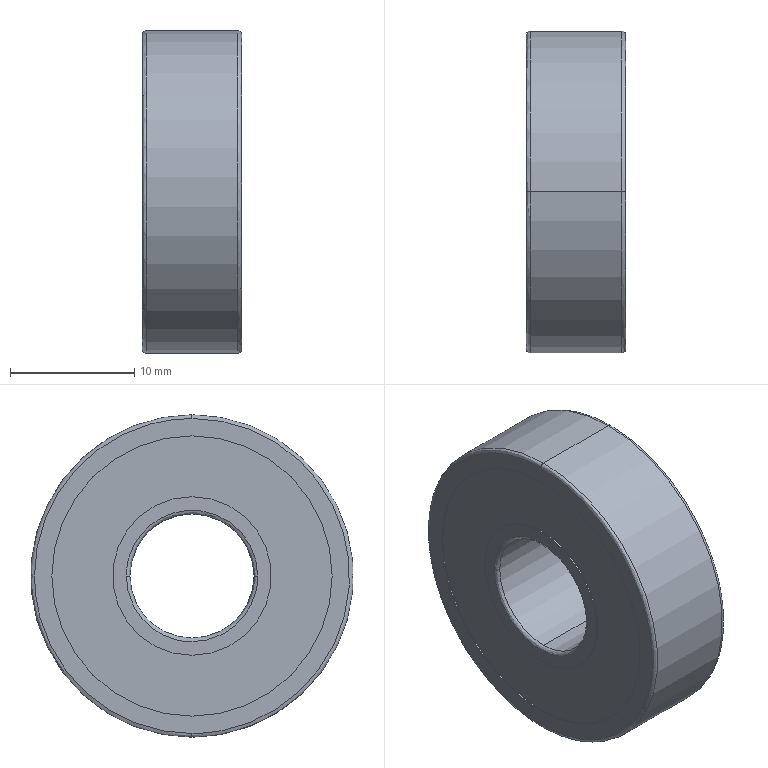Part | STEP file | TQ-DD-1105-TH 6000ZZ_2_031010 Default | 13 solids | 90 faces | box 8 x 26 x 26 mm | volume 2409 mm3 | spline 50 | cylinder 28 | plane 12 | commonest cylinder face diameters 12.8 x8 22.6 x8 14.57 x4 21.45 x4 10 x2 26 x2